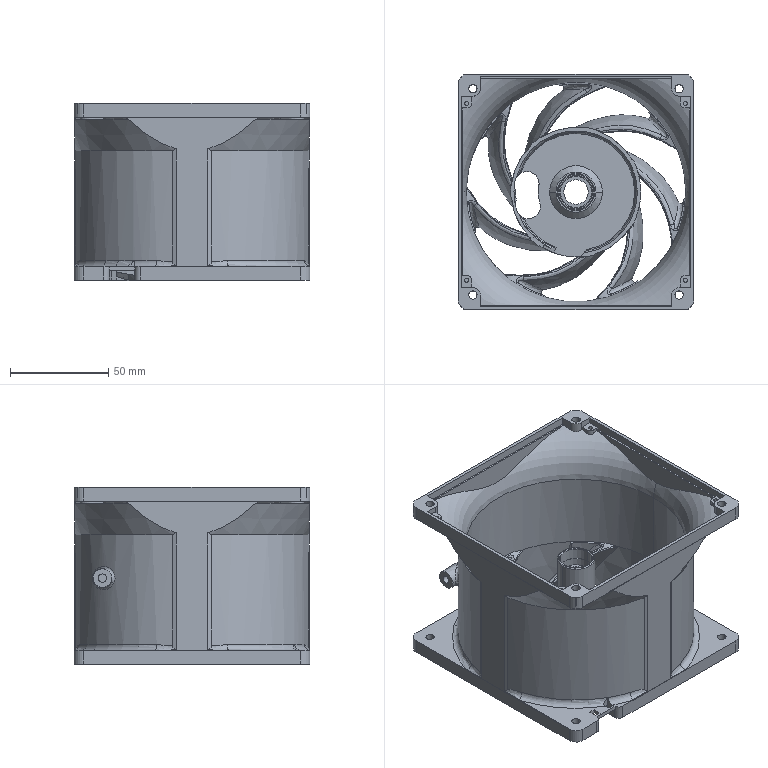NC program | NX | posted with a generic post | part box 120 x 120 x 90.2 mm
Lines 1 to 846 of 828686:
N10 G17 G21 G94 G90
(动态洗_COPY_COPY_1 , TOOL : D12-C)
N12 T02 M6
N14 G54
N16 G17 G0 G90 X-1.189 Y-5.236 S7500 M3
N18 G43 Z113.35 H2
N20 Z95.7
N22 G94 G3 X-1.189 Y-5.236 Z95.108 I1.084 J5.29 F3500.
N24 X-1.189 Y-5.236 Z94.516 I1.084 J5.29
N26 X-1.189 Y-5.236 Z93.923 I1.084 J5.29
N28 X-1.189 Y-5.236 Z93.331 I1.084 J5.29
N30 X-1.189 Y-5.236 Z92.739 I1.084 J5.29
N32 X-1.189 Y-5.236 Z92.147 I1.084 J5.29
N34 X-1.189 Y-5.236 Z91.554 I1.084 J5.29
N36 X-1.189 Y-5.236 Z90.962 I1.084 J5.29
N38 X-1.189 Y-5.236 Z90.37 I1.084 J5.29
N40 X-0.058 Y-5.345 Z90.35 R5.4
N42 X-1.761 Y5.197 R-5.409
N44 X-3.096 Y-4.444 R5.423
N46 X-1.821 Y-5.161 R6.09
N48 X4.142 Y-4.019 R5.646
N50 X5.768 Y-0.896 R5.656
N52 X-1.331 Y5.838 R5.907
N54 X-4.511 Y-3.864 R5.927
N56 X-0.884 Y-5.97 R6.337
N58 X4.486 Y-4.388 R6.157
N60 X6.36 Y0.419 R6.23
N62 X-4.412 Y4.811 R6.434
N64 X-5.528 Y-3.383 R6.459
N66 X-0.255 Y-6.593 R6.806
N68 X4.943 Y-4.68 R6.658
N70 X6.901 Y-0.256 R6.736
N72 X-0.712 Y7.017 R6.963
N74 X-6.56 Y-2.56 R7.005
N76 X0.94 Y-7.134 R7.326
N78 X7.25 Y-1.68 R7.21
N80 X5.152 Y5.522 R7.466
N82 X-3.295 Y6.887 R7.544
N84 X-7.13 Y-2.667 R7.581
N86 X3.882 Y-6.839 R7.867
N88 X7.749 Y-2.038 R7.802
N90 X5.667 Y5.831 R8.03
N92 X-5.06 Y6.486 R8.13
N94 X-7.966 Y-1.959 R8.169
N96 X-1.575 Y-8.141 R8.427
N98 X6.477 Y-5.551 R8.415
N100 X8.123 Y3.076 R8.537
N102 X-4.31 Y7.7 R8.72
N104 X-8.707 Y-1.35 R8.76
N106 X-3.764 Y-8.022 R8.998
N108 X8.823 Y-2.652 R9.035
N110 X7.348 Y5.758 R9.222
N112 X-4.696 Y8.195 R9.343
N114 X-9.194 Y-2.107 R9.397
N116 X-5.261 Y-7.872 R9.601
N118 X9.722 Y-1.643 R9.669
N120 X7.057 Y7.059 R9.877
N122 X-4.295 Y9.116 R9.975
N124 X-9.983 Y-1.332 R10.024
N126 X-3.52 Y-9.511 R10.258
N128 X10.41 Y-1.442 R10.319
N130 X6.766 Y8.209 R10.525
N132 X-6.931 Y8.195 R10.629
N134 X-10.703 Y0.71 R10.66
N136 X-4.957 Y-9.571 R10.876
N138 X9.731 Y-5.339 R10.97
N140 X10.129 Y4.896 R11.094
N142 X-3.932 Y10.686 R11.277
N144 X-11.387 Y0.189 R11.326
N146 X-6.282 Y-9.553 R11.525
N148 X7.632 Y-8.856 R11.637
N150 X11.838 Y-0.579 R11.666
N152 X8.599 Y8.316 R11.843
N154 X-10.97 Y5.047 R11.975
N156 X-8.407 Y-8.694 R12.165
N158 X5.928 Y-10.801 R12.3
N160 X12.545 Y0.153 R12.356
N162 X7.673 Y10.075 R12.552
N164 X-9.16 Y8.892 R12.665
N166 X-12.747 Y-0.521 R12.734
N168 X-6.746 Y-10.89 R12.908
N170 X5.433 Y-11.806 R12.991
N172 X13.224 Y-0.495 R13.05
N174 X8.6 Y10.217 R13.239
N176 X-11.191 Y7.491 R13.356
N178 X-13.19 Y-2.681 R13.497
N180 X-9.072 Y-9.992 R13.626
N182 X6.897 Y-11.862 R13.698
N184 X13.858 Y1.735 R13.773
N186 X7.219 Y12.092 R13.988
N188 X-13.565 Y4.109 R14.072
N190 X-11.93 Y-7.674 R14.265
N192 X-0.72 Y-14.294 R14.359
N194 X13.665 Y-5.126 R14.478
N196 X12.965 Y6.999 R14.567
N198 X-4.477 Y14.189 R14.762
N200 X-14.888 Y0.25 R14.825
N202 X-12.432 Y-8.234 R15.002
N204 X1.353 Y-15.001 R15.089
N206 X15.19 Y2.645 R15.217
N208 X8.499 Y12.991 R15.438
N210 X-14.663 Y5.406 R15.519
N212 X-13.05 Y-8.63 R15.736
N214 X5.199 Y-14.966 R15.83
N216 X15.461 Y4.744 R15.96
N218 X3.01 Y16.025 R16.209
N220 X-16.001 Y3.435 R16.271
N222 X-13.268 Y-9.622 R16.47
N224 X4.951 Y-15.822 R16.573
N226 X15.757 Y6.188 R16.71
N228 X1.541 Y16.99 R16.963
N230 X-16.287 Y5.257 R17.018
N232 X-16.498 Y-4.576 R17.246
N234 X-5.552 Y-16.29 R17.279
N236 X10.857 Y-13.613 R17.383
N238 X16.455 Y6.474 R17.464
N240 X1.829 Y17.718 R17.708
N242 X-17.775 Y1.781 R17.775
N244 X-16.565 Y-6.733 R17.804
N246 X-5.981 Y-16.94 R18.009
N248 X12.347 Y-13.353 R18.144
N250 X17.908 Y-3.934 R18.191
N252 X15.785 Y9.583 R18.251
N254 X3.579 Y18.215 R18.466
N256 X-1.592 Y18.521 R18.263
N258 X-18.209 Y3.935 R18.535
N260 X-15.781 Y-9.961 R18.713
N262 X-3.359 Y-18.453 R18.829
N264 X13.469 Y-13.346 R18.933
N266 X19.068 Y1.944 R18.998
N268 X15.17 Y11.853 R19.076
N270 X2.588 Y19.166 R19.272
N272 X-7.431 Y17.9 R19.413
N274 X-18.912 Y4.322 R19.319
N276 X-9.473 Y-17.021 R19.491
N278 X12.019 Y-15.608 R19.672
N280 X16.715 Y11.01 R19.78
N282 X7.99 Y18.426 R20.001
N284 X1.414 Y20.067 R19.817
N286 X-14.679 Y13.84 R20.068
N288 X-19.978 Y2.813 R20.153
N290 X-8.047 Y-18.603 R20.261
N292 X13.405 Y-15.498 R20.452
N294 X20.618 Y-1.602 R20.537
N296 X18.12 Y10.189 R20.48
N298 X-1.607 Y20.85 R20.805
N300 X-20.468 Y4.493 R20.85
N302 X-20.961 Y0.441 R20.602
N304 X-19.019 Y-8.894 R21.185
N306 X-8.423 Y-19.298 R21.09
N308 X8.009 Y-19.628 R21.191
N310 X21.117 Y-3.717 R21.324
N312 X20.707 Y5.948 R21.335
N314 X11.305 Y18.449 R21.576
N316 X-2.642 Y21.541 R21.552
N318 X-12.292 Y17.928 R21.679
N320 X-21.059 Y5.417 R21.633
N322 X-21.744 Y0.686 R21.099
N324 X-21.454 Y-3.672 R21.481
N326 X-9.94 Y-19.449 R21.804
N328 X3.269 Y-21.695 R21.951
N330 X22.191 Y-1.721 R22.128
N332 X17.403 Y14.083 R22.097
N334 X4.496 Y22.018 R22.376
N336 X-11.809 Y19.185 R22.495
N338 X-21.567 Y6.552 R22.446
N340 X-22.397 Y2.615 R22.336
N342 X-9.375 Y-20.614 R22.618
N344 X3.319 Y-22.491 R22.753
N346 X23.006 Y-1.536 R22.926
N348 X18.838 Y13.508 R22.868
N350 X6.653 Y22.295 R23.213
N352 X-7.353 Y22.12 R23.281
N354 X-15.36 Y17.567 R23.189
N356 X-21.973 Y7.873 R23.285
N358 X-22.857 Y4.762 R23.167
N360 X-10.492 Y-20.969 R23.418
N362 X3.418 Y-23.286 R23.597
N364 X23.861 Y-0.63 R23.726
N366 X19.728 Y13.637 R23.624
N368 X11.539 Y21.095 R24.016
N370 X-1.763 Y24.033 R23.968
N372 X-11.389 Y21.272 R24.117
N374 X-21.217 Y11.526 R24.076
N376 X-24.106 Y1.703 R24.395
N378 X-10.179 Y-22.022 R24.232
N380 X19.623 Y-14.704 R24.496
N382 X23.193 Y8.68 R24.596
N384 X12.567 Y21.441 R24.873
N386 X-2.41 Y24.792 R24.77
N388 X-10.954 Y22.403 R24.774
N390 X-24.082 Y6.582 R24.952
N392 X-8.487 Y-23.602 R25.032
N394 X21.108 Y-14.031 R25.318
N396 X25.304 Y3.374 R25.412
N398 X21.725 Y13.541 R25.071
N400 X-0.941 Y25.702 R25.579
N402 X-6.096 Y25.006 R25.815
N404 X-22.222 Y13.049 R25.726
N406 X-9.982 Y-23.896 R25.843
N408 X22.631 Y-13.156 R26.146
N410 X24.745 Y9.184 R26.237
N412 X17.437 Y19.906 R26.56
N414 X10.481 Y24.341 R26.6
N416 X-8.187 Y25.267 R26.489
N418 X-21.56 Y15.559 R26.506
N420 X-25.93 Y5.983 R26.734
N422 X-7.233 Y-25.735 R26.678
N424 X26.307 Y-6.386 R26.986
N426 X25.358 Y9.89 R27.037
N428 X20.746 Y17.694 R27.453
N430 X11.345 Y24.858 R27.309
N432 X-5.778 Y26.763 R27.366
N434 X-21.963 Y16.402 R27.369
N436 X-27.365 Y2.155 R27.505
N438 X-5.94 Y-26.92 R27.513
N440 X27.957 Y0.406 R27.829
N442 X25.608 Y11.45 R27.694
N444 X20.566 Y19.148 R28.073
N446 X1.293 Y28.153 R28.045
N448 X-11.639 Y25.706 R28.034
N450 X-24.693 Y13.712 R28.164
N452 X-28.259 Y-1.346 R28.175
N454 X-7.162 Y-27.48 R28.34
N456 X28.749 Y1.703 R28.664
N458 X23.578 Y16.734 R28.628
N460 X16.849 Y23.552 R28.887
N462 X12.08 Y26.344 R29.373
N464 X-11.52 Y26.666 R28.965
N466 X-24.662 Y15.402 R29.004
N468 X-28.793 Y-4.465 R29.101
N470 X-6.051 Y-28.606 R29.185
N472 X29.527 Y2.567 R29.506
N474 X22.869 Y19.039 R29.424
N476 X13.85 Y26.395 R29.61
N478 X-2.668 Y29.745 R29.757
N480 X-13.847 Y26.486 R29.709
N482 X-24.14 Y17.663 R29.839
N484 X-26.361 Y14.157 R29.839
N486 X-16.627 Y-25.029 R29.978
N488 X8.757 Y-28.836 R30.159
N490 X30.087 Y4.969 R30.35
N492 X22.962 Y20.228 R30.287
N494 X15.152 Y26.63 R30.357
N496 X-0.718 Y30.69 R30.546
N498 X-16.621 Y25.847 R30.61
N500 X-27.683 Y13.426 R30.804
N502 X-15.705 Y-26.607 R30.824
N504 X9.975 Y-29.334 R31.005
N506 X29.185 Y11.545 R31.206
N508 X21.38 Y23.077 R31.186
N510 X-10.154 Y29.885 R31.462
N512 X-19.687 Y-24.888 R31.656
N514 X10.823 Y-29.935 R31.831
N516 X29.904 Y12.019 R32.058
N518 X18.2 Y26.706 R31.978
N520 X0.031 Y32.385 R32.248
N522 X-17.116 Y27.53 R32.31
N524 X-26.655 Y18.499 R32.446
N526 X-22.964 Y-23.102 R32.493
N528 X11.318 Y-30.659 R32.664
N530 X30.672 Y12.38 R32.912
N532 X21.099 Y25.578 R32.743
N534 X-17.41 Y28.345 R33.137
N536 X-33.275 Y2.262 R33.334
N538 X-14.706 Y-30.048 R33.385
N540 X15.28 Y-29.871 R33.573
N542 X31.481 Y12.646 R33.767
N544 X22.245 Y25.724 R33.627
N546 X-9.007 Y32.894 R34.004
N548 X-34.189 Y-1.433 R34.21
N550 X-9.111 Y-33.095 R34.267
N552 X19.272 Y-28.526 R34.46
N554 X33.026 Y10.847 R34.614
N556 X23.838 Y25.43 R34.416
N558 X8.501 Y33.863 R34.763
N560 X-19.103 Y29.294 R34.832
N562 X-28.698 Y-20.258 R35.043
N564 X9.004 Y-34.068 R35.209
N566 X33.582 Y-11.339 R35.523
N568 X28.738 Y21.166 R35.515
N570 X-5.548 Y35.378 R35.714
N572 X-31.006 Y18.051 R35.923
N574 X-21.633 Y-28.793 R35.928
N576 X19.509 Y-30.421 R36.121
N578 X35.881 Y-5.795 R36.365
N580 X28.985 Y22.27 R36.374
N582 X5.102 Y36.288 R36.568
N584 X-16.464 Y32.783 R36.562
N586 X-22.633 Y28.89 R36.534
N588 X-35.485 Y9.629 R36.719
N590 X-21.66 Y-29.849 R36.794
N592 X20.505 Y-30.805 R36.987
N594 X36.239 Y-8.345 R37.259
N596 X29.218 Y23.376 R37.235
N598 X-4.456 Y37.263 R37.417
N600 X-26.493 Y26.646 R37.621
N602 X-35.78 Y11.648 R37.56
N604 X-23.639 Y-29.422 R37.653
N606 X19.427 Y-32.502 R37.846
N608 X36.007 Y-12.212 R38.18
N610 X33.707 Y18.063 R38.114
N612 X23.476 Y30.275 R37.878
N614 X11.015 Y36.739 R38.186
N616 X-10.826 Y36.845 R38.21
N618 X-23.799 Y30.175 R38.457
N620 X-38.253 Y4.53 R38.477
N622 X-17.815 Y-34.273 R38.553
N624 X24.991 Y-29.624 R38.745
N626 X36.865 Y-12.378 R39.075
N628 X29.574 Y25.661 R38.969
N630 X-1.427 Y39.229 R39.155
N632 X-28.761 Y26.808 R39.355
N634 X-30.487 Y-25.061 R39.365
N636 X12.72 Y-37.478 R39.552
N638 X32.011 Y-23.436 R39.805
N640 X36.403 Y16.471 R39.817
N642 X19.793 Y34.836 R39.704
N644 X-13.816 Y37.692 R40.022
N646 X-32.715 Y23.369 R40.282
N648 X-28.849 Y-28.204 R40.246
N650 X16.282 Y-37.041 R40.439
N652 X34.542 Y-21.261 R40.704
N654 X37.334 Y16.513 R40.687
N656 X20.759 Y35.281 R40.568
N658 X-12.355 Y39.108 R40.871
N660 X-40.146 Y8.933 R41.118
N662 X-22.519 Y-34.547 R41.157
N664 X24.506 Y-33.327 R41.349
N666 X40.818 Y-7.67 R41.67
N668 X30.757 Y28.265 R41.602
N670 X-10.666 Y40.502 R41.751
N672 X-33.622 Y-25.315 R41.98
N674 X11.969 Y-40.465 R42.171
N676 X37.036 Y-20.476 R42.385
N678 X37.694 Y19.817 R42.46
N680 X25.769 Y34.011 R42.191
N682 X-10.191 Y41.525 R42.617
N684 X-35.085 Y-24.798 R42.855
N686 X11.017 Y-41.641 R43.045
N688 X38.029 Y-20.492 R43.25
N690 X31.056 Y30.501 R43.341
N692 X-11.58 Y42.073 R43.513
N694 X-43.788 Y0.199 R43.732
N696 X-15.731 Y-40.977 R43.827
N698 X32.036 Y-30.207 R44.02
N700 X44.158 Y-1.839 R44.306
N702 X32.239 Y30.534 R44.242
N704 X10.679 Y43.178 R44.326
N706 X-16.263 Y41.451 R44.509
N708 X-37.834 Y-23.849 R44.61
N710 X8.982 Y-43.922 R44.8
N712 X40.677 Y-19.175 R44.994
N714 X31.396 Y32.647 R45.113
N716 X-8.87 Y44.517 R45.244
N718 X-35.223 Y28.755 R45.481
N720 X-39.259 Y-23.209 R45.49
N722 X7.943 Y-45.017 R45.681
N724 X42.409 Y-17.464 R45.871
N726 X30.737 Y34.471 R46.002
N728 X-10.624 Y45.043 R46.157
N730 X-44.658 Y12.637 R46.379
N732 X-27.536 Y-37.501 R46.438
N734 X25.547 Y-39.032 R46.631
N736 X44.343 Y-14.852 R46.848
N738 X31.207 Y35.238 R46.898
N740 X-9.366 Y46.223 R47.034
N742 X-42.267 Y-21.397 R47.257
N744 X5.329 Y-47.18 R47.445
N746 X44.782 Y-16.268 R47.638
N748 X31.465 Y36.193 R47.792
N750 X-10.783 Y46.826 R47.923
N752 X-44.657 Y18.072 R48.148
N754 X-32.753 Y-35.489 R48.198
N756 X21.683 Y-43.284 R48.391
N758 X47.399 Y-10.565 R48.586
N760 X32.19 Y36.736 R48.677
N762 X-8.236 Y48.237 R48.789
N764 X-44.682 Y-20.479 R49.031
N766 X3.473 Y-49.133 R49.219
N768 X47.377 Y-14.117 R49.411
N770 X32.435 Y37.704 R49.585
N772 X-8.132 Y49.158 R49.684
N774 X-45.805 Y-20.155 R49.921
N776 X2.862 Y-50.066 R50.109
N778 X48.06 Y-14.931 R50.302
N780 X34.075 Y37.435 R50.503
N782 X10.604 Y49.566 R50.477
N784 X-16.393 Y48.013 R50.745
N786 X-48.26 Y-16.273 R50.804
N788 X-1.867 Y-50.998 R50.989
N790 X47.301 Y-19.606 R51.182
N792 X39.784 Y32.664 R51.411
N794 X30.011 Y41.893 R51.077
N796 X-10.255 Y50.584 R51.486
N798 X-49.401 Y-15.663 R51.697
N800 X-2.743 Y-51.854 R51.882
N802 X47.705 Y-20.932 R52.075
N804 X38.094 Y35.959 R52.307
N806 X22.514 Y47.372 R51.944
N808 X-10.015 Y51.543 R52.389
N810 X-41.437 Y32.413 R52.607
N812 X-43.756 Y-29.453 R52.632
N814 X12.281 Y-51.408 R52.825
N816 X52.638 Y-6.593 R53.018
N818 X33.655 Y41.346 R53.199
N820 X-2.082 Y53.35 R53.209
N822 X-39.833 Y35.712 R53.534
N824 X-45.517 Y-28.383 R53.526
N826 X10.764 Y-52.661 R53.719
N828 X53.292 Y-8.348 R53.912
N830 X37.52 Y39.096 R54.12
N832 X10.469 Y53.249 R53.919
N834 X-14.326 Y52.389 R54.37
N836 X-40.827 Y35.948 R54.393
N838 X-47.011 Y-27.649 R54.421
N840 X9.337 Y-53.842 R54.614
N842 X53.918 Y-9.989 R54.807
N844 X37.64 Y40.225 R55.033
N846 X14.097 Y53.33 R54.819
N848 X-13.5 Y53.533 R55.245
N850 X-54.585 Y-9.512 R55.277
N852 X-10.223 Y-54.561 R55.457
N854 X47.646 Y-28.789 R55.65
N856 X53.703 Y15.299 R55.854
N858 X34.309 Y44.272 R55.865
N860 X-2.543 Y56.029 R55.913
N862 X-41.347 Y38.061 R56.225
N864 X-48.24 Y-29.111 R56.226
N866 X10.182 Y-55.524 R56.418
N868 X55.772 Y-9.876 R56.611
N870 X39.926 Y40.513 R56.849
N872 X16.08 Y54.642 R56.547
N874 X-12.281 Y55.668 R57.044
N876 X-56.764 Y-7.122 R57.074
N878 X-13.316 Y-55.743 R57.255
N880 X47.613 Y-32.174 R57.448
N882 X53.577 Y21.33 R57.64
N884 X31.682 Y48.376 R57.639
N886 X-5.213 Y57.657 R57.758
N888 X-57.832 Y-5.681 R57.975
N890 X-14.915 Y-56.27 R58.156
N892 X47.618 Y-33.75 R58.349
N894 X53.781 Y23.215 R58.536
N896 X32.722 Y48.767 R58.552
N898 X7.292 Y58.325 R58.561
N900 X-28.481 Y51.51 R58.993
N902 X-58.762 Y-5.466 R58.879
N904 X-15.643 Y-57.012 R59.06
N906 X48.137 Y-34.58 R59.253
N908 X53.536 Y25.947 R59.441
N910 X33.569 Y49.285 R59.506
N912 X2.178 Y59.65 R59.489
N914 X-38.956 Y45.371 R59.841
N916 X-53.84 Y-26.381 R59.832
N918 X-51.183 Y-31.239 R59.428
N920 X-16.677 Y-57.665 R59.966
N922 X-11.884 Y-58.847 R60.221
N924 X-9.471 Y-59.282 R124.09
N926 X-2.449 Y-60. R59.485
N928 G1 X2.051
N930 G3 X11.802 Y-58.904 R58.047
N932 X14.142 Y-58.388 R107.122
N934 X53.022 Y-28.515 R60.183
N936 X58.831 Y-13.024 R60.298
N938 X59.263 Y-10.909 R126.002
N940 X60. Y-5.804 R59.599
N942 G1 Y4.571
N944 G3 X59.571 Y9.376 R41.526
N946 X58.834 Y13.392 R50.986
N948 X58.141 Y16.194 R75.005
N950 X45.195 Y40.189 R60.446
N952 X19.942 Y57.199 R60.08
N954 X14.362 Y58.858 R60.474
N956 X12.183 Y59.346 R125.01
N958 X8.513 Y59.99 R58.988
N960 G1 X8.374 Y60.
N962 X-6.626
N964 G3 X-10.464 Y59.644 R30.891
N966 X-15.042 Y58.718 R46.197
N968 X-28.099 Y53.774 R59.232
N970 X-58.863 Y15.209 R60.676
N972 X-59.409 Y12.919 R111.397
N974 X-59.988 Y9.927 R56.713
N976 G1 X-60. Y9.782
N978 Y-7.968
N980 G3 X-59.666 Y-11.393 R26.915
N982 X-58.711 Y-15.886 R43.567
N984 X-54.846 Y-26.392 R58.44
N986 X-15.742 Y-58.873 R60.892
N988 X-13.274 Y-59.476 R89.912
N990 X-10.857 Y-59.969 R62.855
N992 X-10.588 Y-60. R2.057
N994 G1 X8.801
N996 G3 X11.748 Y-59.713 R24.221
N998 X16.418 Y-58.708 R41.927
N1000 X25.62 Y-55.374 R57.748
N1002 X58.847 Y-16.648 R61.155
N1004 X59.531 Y-14.018 R97.113
N1006 X59.964 Y-12.072 R62.148
N1008 X60. Y-11.791 R2.049
N1010 G1 Y-5.791
N1012 Y-13.791
N1014 G2 X59.711 Y-16.093 R16.354
N1016 X58.756 Y-19.751 R30.681
N1018 X56.236 Y-26.175 R53.255
N1020 X32.565 Y-52.692 R61.925
N1022 X19.233 Y-58.829 R60.701
N1024 X17.003 Y-59.487 R86.005
N1026 X15.055 Y-59.976 R41.658
N1028 G1 X14.858 Y-60.
N1030 X8.733
N1032 X16.358
N1034 G3 X18.068 Y-59.805 R12.259
N1036 X20.942 Y-59.092 R25.181
N1038 X22.307 Y-58.638 R34.625
N1040 X28.346 Y-56.076 R51.209
N1042 X41.034 Y-47.648 R62.501
N1044 X56.746 Y-27.228 R62.785
N1046 X58.821 Y-22.341 R56.295
N1048 X59.503 Y-20.349 R74.843
N1050 X59.954 Y-18.825 R36.565
N1052 X60. Y-18.516 R1.974
N1054 G1 Y-13.766
N1056 Y-19.641
N1058 G2 X59.734 Y-21.486 R10.945
N1060 X58.746 Y-24.694 R23.093
N1062 X56.572 Y-29.558 R44.989
N1064 X50.245 Y-39.356 R61.55
N1066 X29.738 Y-56.39 R63.483
N1068 X24.253 Y-58.88 R54.746
N1070 X21.76 Y-59.752 R45.638
N1072 G1 X21.338 Y-59.881
N1074 G2 X20.782 Y-60. R2.36
N1076 G1 X16.282
N1078 X21.782
N1080 G3 X23.375 Y-59.772 R9.747
N1082 X26.526 Y-58.783 R21.437
N1084 X30.909 Y-56.768 R42.052
N1086 X39.264 Y-51.422 R60.643
N1088 X56.078 Y-32.368 R64.133
N1090 X58.899 Y-26.712 R51.43
N1092 X59.779 Y-24.387 R38.225
N1094 X59.953 Y-23.837 R9.397
N1096 X60. Y-23.527 R1.969
N1098 G1 Y-19.527
N1100 Y-24.402
N1102 G2 X59.779 Y-25.834 R8.645
N1104 X58.73 Y-28.937 R18.664
N1106 X56.744 Y-32.959 R39.112
N1108 X52.154 Y-39.881 R59.122
N1110 X34.474 Y-55.793 R64.695
N1112 X28.944 Y-58.726 R50.979
N1114 X26.522 Y-59.702 R40.058
N1116 X25.801 Y-59.946 R19.808
N1118 X25.416 Y-60. R1.699
N1120 G1 X21.666
N1122 X26.166
N1124 G3 X27.417 Y-59.835 R7.312
N1126 X29.778 Y-59.106 R15.973
N1128 X33.033 Y-57.599 R32.026
N1130 X38.242 Y-54.414 R51.962
N1132 X55.705 Y-36.433 R64.884
N1134 X58.616 Y-31.311 R48.721
N1136 X59.811 Y-28.503 R30.019
N1138 X59.955 Y-28.071 R5.51
N1140 X60. Y-27.767 R1.986
N1142 G1 Y-24.392
N1144 Y-28.517
N1146 G2 X59.768 Y-29.874 R7.659
N1148 X58.799 Y-32.545 R16.392
N1150 X56.974 Y-36.018 R33.568
N1152 X53.212 Y-41.494 R54.768
N1154 X37.982 Y-55.693 R65.005
N1156 X33.262 Y-58.477 R47.72
N1158 X30.316 Y-59.786 R29.487
N1160 G1 X30.027 Y-59.89
N1162 G2 X29.505 Y-60. R1.756
N1164 G1 X26.13
N1166 X30.13
N1168 G3 X31.431 Y-59.799 R6.704
N1170 X33.664 Y-59.028 R14.857
N1172 X37.146 Y-57.225 R31.3
N1174 X42.13 Y-53.821 R51.691
N1176 X55.497 Y-39.943 R64.683
N1178 X58.358 Y-35.38 R46.303
N1180 X59.703 Y-32.545 R28.227
N1182 X59.917 Y-31.982 R18.13
N1184 X60. Y-31.549 R1.782
N1186 G1 Y-28.424
N1188 Y-32.174
N1190 G2 X59.857 Y-33.134 R5.698
N1192 X59.218 Y-35.083 R12.449
N1194 X57.83 Y-37.855 R24.639
N1196 X55.239 Y-41.798 R43.125
N1198 X46.735 Y-51.176 R62.864
N1200 X40.282 Y-56.286 R61.317
N1202 X36.274 Y-58.719 R40.773
N1204 X34.048 Y-59.75 R26.131
N1206 X33.534 Y-59.941 R8.971
N1208 X33.143 Y-60. R1.853
N1210 G1 X30.018
N1212 X33.768
N1214 G3 X35.069 Y-59.77 R6.536
N1216 X37.096 Y-59.017 R13.715
N1218 X40.446 Y-57.167 R28.328
N1220 X44.877 Y-53.956 R48.912
N1222 X55.631 Y-42.794 R62.602
N1224 X58.337 Y-38.719 R42.559
N1226 X59.679 Y-36.054 R24.963
N1228 X59.938 Y-35.388 R9.894
N1230 X60. Y-34.993 R1.85
N1232 G1 Y-32.118
N1234 Y-35.618
N1236 G2 X59.825 Y-36.646 R6.035
N1238 X59.115 Y-38.602 R12.192
N1240 X57.828 Y-41.009 R23.321
N1242 X55.233 Y-44.746 R40.062
N1244 X48.55 Y-51.991 R59.905
N1246 X43.038 Y-56.494 R57.349
N1248 X39.325 Y-58.837 R35.948
N1250 X36.976 Y-59.925 R19.212
N1252 X36.56 Y-60. R1.817
N1254 G1 X33.685
N1256 X37.06
N1258 G3 X38.149 Y-59.825 R5.655
N1260 X39.884 Y-59.206 R11.292
N1262 X42.032 Y-58.085 R20.905
N1264 X45.511 Y-55.715 R36.05
N1266 X52.467 Y-49.384 R56.997
N1268 X56.652 Y-44.352 R54.177
N1270 X58.83 Y-40.984 R33.752
N1272 X59.894 Y-38.767 R19.053
N1274 X60. Y-38.25 R1.742
N1276 G1 Y-35.5
N1278 Y-38.75
N1280 G2 X59.832 Y-39.783 R5.245
N1282 X59.072 Y-41.789 R11.48
N1284 X57.902 Y-43.884 R21.972
N1286 X55.417 Y-47.338 R36.365
N1288 X46.331 Y-56.215 R54.829
N1290 X42.798 Y-58.62 R35.289
N1292 X40.622 Y-59.733 R20.613
N1294 X40.127 Y-59.932 R7.379
N1296 X39.723 Y-60. R1.838
N1298 G1 X36.973
N1300 X40.223
N1302 G3 X41.498 Y-59.758 R5.706
N1304 X43.471 Y-58.947 R12.322
N1306 X46.581 Y-57.032 R25.282
N1308 X50.854 Y-53.531 R44.157
N1310 X56.399 Y-47.533 R50.975
N1312 X58.695 Y-44.21 R32.698
N1314 X59.894 Y-41.833 R17.799
N1316 X60. Y-41.316 R1.743
N1318 G1 Y-38.691
N1320 Y-41.816
N1322 G2 X59.857 Y-42.686 R5.043
N1324 X59.3 Y-44.249 R9.492
N1326 X58.362 Y-46.019 R17.222
N1328 X56.293 Y-48.983 R28.619
N1330 X51.203 Y-54.418 R45.977
N1332 X47.201 Y-57.654 R40.858
N1334 X44.696 Y-59.213 R24.69
N1336 X43.181 Y-59.922 R14.726
N1338 X42.759 Y-60. R1.806
N1340 G1 X40.134
N1342 X43.259
N1344 G3 X44.547 Y-59.73 R5.663
N1346 X46.327 Y-58.966 R11.931
N1348 X49.177 Y-57.16 R23.022
N1350 X53.513 Y-53.416 R38.813
N1352 X57.353 Y-49.026 R40.189
N1354 X59.09 Y-46.391 R24.903
N1356 X59.885 Y-44.776 R15.361
N1358 X60. Y-44.248 R1.741
N1360 G1 Y-41.748
N1362 Y-44.748
N1364 G2 X59.844 Y-45.62 R4.973
N1366 X59.252 Y-47.183 R9.342
N1368 X58.394 Y-48.738 R16.729
N1370 X56.244 Y-51.686 R26.104
N1372 X50.345 Y-57.351 R37.293
N1374 X47.735 Y-59.098 R23.894
N1376 X46.136 Y-59.893 R14.935
N1378 X45.617 Y-60. R1.742
N1380 G1 X43.242
N1382 X46.117
N1384 G3 X46.982 Y-59.844 R4.798
N1386 X48.486 Y-59.271 R9.105
N1388 X50.05 Y-58.397 R16.057
N1390 X52.958 Y-56.23 R25.062
N1392 X57.523 Y-51.439 R32.788
N1394 X58.854 Y-49.526 R23.385
N1396 X59.828 Y-47.694 R16.257
N1398 X60. Y-47.042 R1.729
N1400 G1 Y-44.667
N1402 Y-47.417
N1404 G2 X59.862 Y-48.286 R4.233
N1406 X59.288 Y-49.801 R8.729
N1408 X58.435 Y-51.307 R14.651
N1410 X56.128 Y-54.293 R23.139
N1412 X51.859 Y-58.148 R27.727
N1414 X49.44 Y-59.626 R17.291
N1416 X48.834 Y-59.904 R12.06
N1418 X48.326 Y-60. R1.669
N1420 G1 X46.076
N1422 X48.826
N1424 G3 X49.69 Y-59.834 R4.748
N1426 X51.289 Y-59.18 R8.958
N1428 X53.201 Y-57.989 R15.614
N1430 X56.994 Y-54.523 R23.412
N1432 X58.828 Y-52.133 R21.122
N1434 X59.742 Y-50.508 R15.092
N1436 G1 X59.846 Y-50.283
N1438 G3 X60. Y-49.654 R1.622
N1440 G1 Y-47.404
N1442 Y-50.154
N1444 G2 X59.824 Y-51.015 R4.696
N1446 X59.21 Y-52.487 R8.425
N1448 X57.725 Y-54.737 R14.753
N1450 X53.486 Y-58.724 R20.021
N1452 X51.658 Y-59.784 R13.855
N1454 X51.304 Y-59.933 R2.988
N1456 X50.901 Y-60. R1.841
N1458 G1 X48.776
N1460 X51.276
N1462 G3 X52.103 Y-59.857 R4.145
N1464 X53.663 Y-59.206 R7.779
N1466 X55.319 Y-58.128 R12.893
N1468 X58.907 Y-54.368 R16.656
N1470 X59.751 Y-52.927 R13.606
N1472 X59.924 Y-52.536 R3.885
N1474 X60. Y-52.117 R1.813
N1476 G1 Y-50.117
N1478 Y-52.492
N1480 G2 X59.837 Y-53.341 R4.027
N1482 X59.215 Y-54.77 R7.398
N1484 X58.432 Y-55.963 R11.53
N1486 X54.917 Y-59.251 R13.611
N1488 X53.795 Y-59.871 R9.959
N1490 X53.246 Y-60. R1.69
N1492 G1 X51.246
N1494 X53.621
N1496 G3 X54.389 Y-59.85 R3.692
N1498 X55.813 Y-59.205 R6.921
N1500 X57.611 Y-57.83 R9.433
N1502 X59.114 Y-56.102 R12.821
N1504 X59.881 Y-54.816 R8.986
N1506 X60. Y-54.283 R1.737
N1508 G1 Y-52.408
N1510 Y-54.658
N1512 G2 X59.882 Y-55.26 R3.508
N1514 X59.451 Y-56.292 R5.573
N1516 X57.639 Y-58.588 R8.759
N1518 X55.851 Y-59.843 R8.334
N1520 X55.372 Y-59.976 R1.547
N1522 G1 X55.307 Y-59.987
N1524 X55.028 Y-59.999
N1526 X54.972 Y-60.
N1528 X53.597
N1530 X54.972
N1532 X55.028 Y-59.999
N1534 X55.307 Y-59.987
N1536 G3 X56.585 Y-59.738 R4.834
N1538 X58.184 Y-58.722 R6.227
N1540 X59.256 Y-57.588 R7.626
N1542 X59.41 Y-57.347 R2.605
N1544 X59.842 Y-56.24 R4.926
N1546 X59.999 Y-55.028 R5.294
N1548 G1 X60. Y-54.597
N1550 G2 X59.974 Y-55.49 R8.728
N1552 X59.506 Y-57.162 R5.066
N1554 G1 X59.41 Y-57.347
N1556 G2 X59.062 Y-57.912 R4.754
N1558 X56.658 Y-59.715 R5.023
N1560 G1 X56.538 Y-59.753
N1562 G2 X55.074 Y-59.081 R1.2
N1564 G1 X55.05 Y-59.018 Z90.364
N1566 X55.029 Y-58.954 Z90.378
N1568 X55.011 Y-58.889 Z90.393
N1570 X54.997 Y-58.824 Z90.407
N1572 X54.987 Y-58.757 Z90.421
N1574 X54.98 Y-58.69 Z90.435
N1576 X54.978 Y-58.623 Z90.45
N1578 X54.979 Y-58.556 Z90.464
N1580 X54.983 Y-58.489 Z90.478
N1582 X54.992 Y-58.422 Z90.492
N1584 X55.004 Y-58.356 Z90.506
N1586 X55.02 Y-58.291 Z90.521
N1588 X55.04 Y-58.226 Z90.535
N1590 X55.063 Y-58.163 Z90.549
N1592 X55.09 Y-58.101 Z90.563
N1594 X55.12 Y-58.041 Z90.578
N1596 X55.729 Y-56.906 Z90.85
N1598 X56.425 Y-55.602 F15000.
N1600 G3 X56.538 Y-55.097 R1.209
N1602 G1 X56.71 Y1.345
N1604 G2 X57.04 Y2.105 R1.201
N1606 G1 X57.088 Y2.152 Z90.836 F3500.
N1608 X57.139 Y2.197 Z90.821
N1610 X57.192 Y2.239 Z90.807
N1612 X57.247 Y2.278 Z90.793
N1614 X59.057 Y3.333 Z90.35
N1616 G3 X59.514 Y3.607 R6.983
N1618 X60. Y4.571 R1.2
N1620 G1 Y10.196
N1622 G3 X59.737 Y12.794 R21.882
N1624 X58.728 Y17.328 R38.686
N1626 X55.721 Y25.568 R56.825
N1628 X41.43 Y45.343 R61.336
N1630 X17.92 Y58.823 R61.105
N1632 X15.251 Y59.569 R92.884
N1634 X13.56 Y59.977 R49.179
N1636 G1 X13.369 Y60.
N1638 X8.369
N1640 X14.994
N1642 G2 X17.272 Y59.704 R14.785
N1644 X20.817 Y58.735 R28.59
N1646 X26.781 Y56.335 R51.528
N1648 X41.819 Y46.225 R61.531
N1650 X57.642 Y23.379 R62.172
N1652 X59.847 Y16.627 R55.071
N1654 G1 X59.946 Y16.227
N1656 G2 X60. Y15.843 R1.697
N1658 G1 Y10.093
N1660 Y17.343
N1662 G3 X59.75 Y19.242 R12.671
N1664 X58.759 Y22.755 R26.624
N1666 X56.433 Y28.293 R49.252
N1668 X48.85 Y40.108 R62.227
N1670 X36.419 Y51.741 R62.481
N1672 X25.389 Y57.961 R60.84
N1674 X20.552 Y59.753 R47.622
N1676 G1 X19.97 Y59.925
N1678 G3 X19.553 Y60. R1.816
N1680 G1 X14.928
N1682 X20.553
N1684 G2 X22.166 Y59.786 R9.723
N1686 X25.429 Y58.792 R21.669
N1688 X29.813 Y56.826 R42.548
N1690 X38.399 Y51.426 R60.134